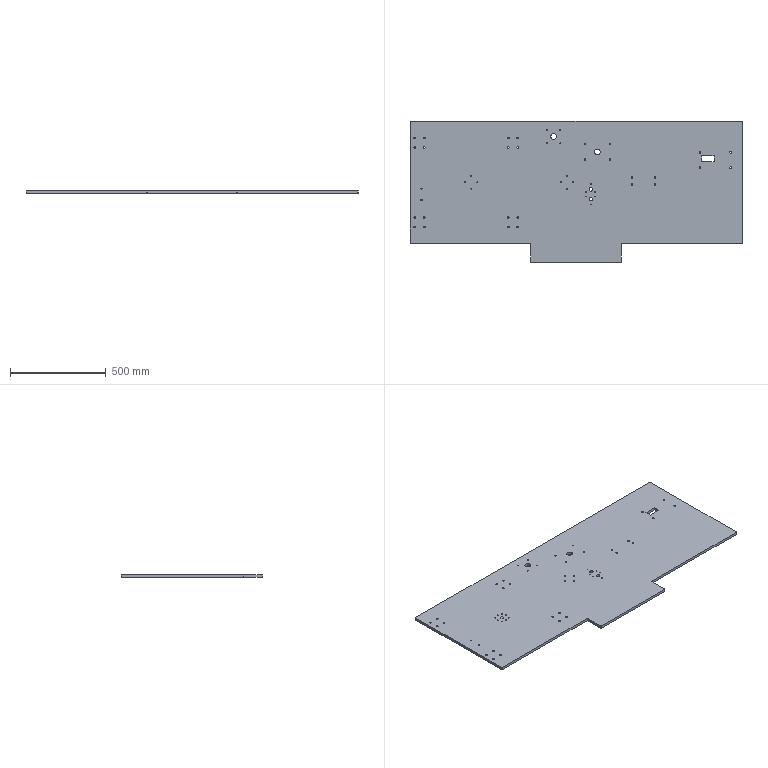Part | STEP file | Double-tube top plate SGN-1-04 | 1 solid | 143 faces | box 1734 x 739 x 14 mm | volume 16088539 mm3 | cylinder 120 | plane 15 | cone 8 | commonest cylinder face diameters 9 x48 4.2 x28 5 x16 6.8 x12 6 x6 18 x4